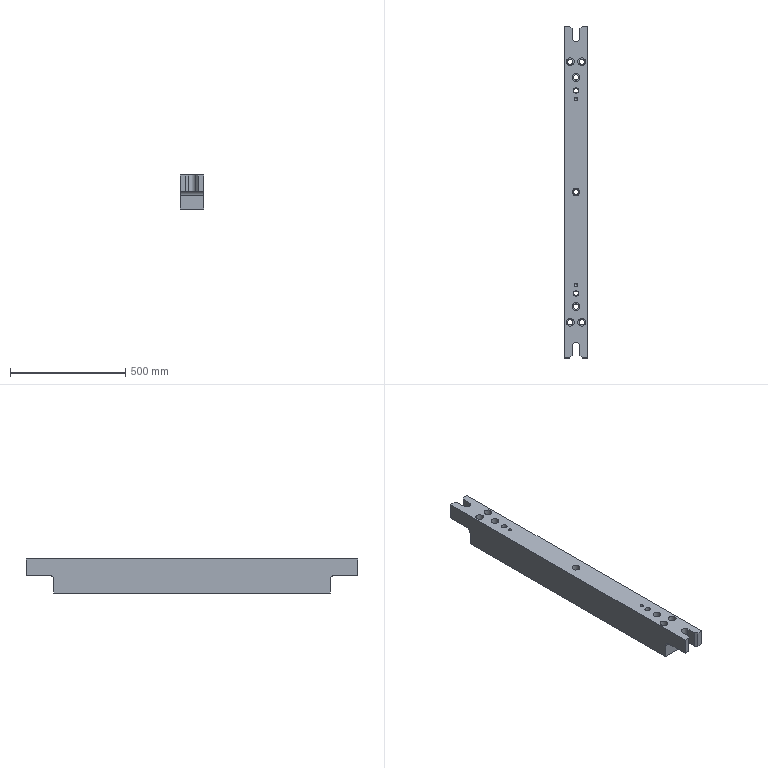Part | STEP file | lll_id1770_x_t | 1 solid | 55 faces | box 100 x 1440 x 147.5 mm | volume 18182535 mm3 | plane 29 | cylinder 24 | cone 2 | commonest cylinder face diameters 23.009 x7 34.008 x7 14.506 x2 20 x2 24 x2 34 x2
STEP:
#1=CARTESIAN_POINT('',(2475.431,565.,370.));
#2=VERTEX_POINT('',#1);
#3=CARTESIAN_POINT('',(2492.435,565.,370.));
#4=DIRECTION('',(0.,0.,-1.));
#5=DIRECTION('',(-1.,0.,0.));
#6=AXIS2_PLACEMENT_3D('',#3,#4,#5);
#7=CIRCLE('',#6,17.004);
#8=EDGE_CURVE('',#2,#2,#7,.T.);
#9=ORIENTED_EDGE('',*,*,#8,.T.);
#10=EDGE_LOOP('',(#9));
#11=FACE_BOUND('',#10,.T.);
#12=CARTESIAN_POINT('',(2505.435,440.,370.));
#13=VERTEX_POINT('',#12);
#14=CARTESIAN_POINT('',(2517.435,440.,370.));
#15=DIRECTION('',(0.,0.,-1.));
#16=DIRECTION('',(-1.,0.,0.));
#17=AXIS2_PLACEMENT_3D('',#14,#15,#16);
#18=CIRCLE('',#17,12.);
#19=EDGE_CURVE('',#13,#13,#18,.T.);
#20=ORIENTED_EDGE('',*,*,#19,.T.);
#21=EDGE_LOOP('',(#20));
#22=FACE_BOUND('',#21,.T.);
#23=CARTESIAN_POINT('',(2500.431,497.,370.));
#24=VERTEX_POINT('',#23);
#25=CARTESIAN_POINT('',(2517.435,497.,370.));
#26=DIRECTION('',(0.,0.,-1.));
#27=DIRECTION('',(-1.,0.,0.));
#28=AXIS2_PLACEMENT_3D('',#25,#26,#27);
#29=CIRCLE('',#28,17.004);
#30=EDGE_CURVE('',#24,#24,#29,.T.);
#31=ORIENTED_EDGE('',*,*,#30,.T.);
#32=EDGE_LOOP('',(#31));
#33=FACE_BOUND('',#32,.T.);
#34=CARTESIAN_POINT('',(2525.431,565.,370.));
#35=VERTEX_POINT('',#34);
#36=CARTESIAN_POINT('',(2542.435,565.,370.));
#37=DIRECTION('',(0.,0.,-1.));
#38=DIRECTION('',(-1.,0.,0.));
#39=AXIS2_PLACEMENT_3D('',#36,#37,#38);
#40=CIRCLE('',#39,17.004);
#41=EDGE_CURVE('',#35,#35,#40,.T.);
#42=ORIENTED_EDGE('',*,*,#41,.T.);
#43=EDGE_LOOP('',(#42));
#44=FACE_BOUND('',#43,.T.);
#45=CARTESIAN_POINT('',(2534.439,0.,370.));
#46=VERTEX_POINT('',#45);
#47=CARTESIAN_POINT('',(2517.435,0.,370.));
#48=DIRECTION('',(0.,0.,-1.));
#49=DIRECTION('',(1.,0.,0.));
#50=AXIS2_PLACEMENT_3D('',#47,#48,#49);
#51=CIRCLE('',#50,17.004);
#52=EDGE_CURVE('',#46,#46,#51,.T.);
#53=ORIENTED_EDGE('',*,*,#52,.T.);
#54=EDGE_LOOP('',(#53));
#55=FACE_BOUND('',#54,.T.);
#56=CARTESIAN_POINT('',(2534.439,-497.,370.));
#57=VERTEX_POINT('',#56);
#58=CARTESIAN_POINT('',(2517.435,-497.,370.));
#59=DIRECTION('',(0.,0.,1.));
#60=DIRECTION('',(1.,0.,0.));
#61=AXIS2_PLACEMENT_3D('',#58,#59,#60);
#62=CIRCLE('',#61,17.004);
#63=EDGE_CURVE('',#57,#57,#62,.T.);
#64=ORIENTED_EDGE('',*,*,#63,.F.);
#65=EDGE_LOOP('',(#64));
#66=FACE_BOUND('',#65,.T.);
#67=CARTESIAN_POINT('',(2534.435,-710.,370.));
#68=VERTEX_POINT('',#67);
#69=CARTESIAN_POINT('',(2534.435,-670.,370.));
#70=VERTEX_POINT('',#69);
#71=CARTESIAN_POINT('',(2534.435,120.,370.));
#72=DIRECTION('',(0.,1.,0.));
#73=VECTOR('',#72,1.);
#74=LINE('',#71,#73);
#75=EDGE_CURVE('',#68,#70,#74,.T.);
#76=ORIENTED_EDGE('',*,*,#75,.F.);
#77=CARTESIAN_POINT('',(2544.435,-720.,370.));
#78=VERTEX_POINT('',#77);
#79=CARTESIAN_POINT('',(2534.435,-710.,370.));
#80=DIRECTION('',(0.7071,-0.7071,0.));
#81=VECTOR('',#80,1.);
#82=LINE('',#79,#81);
#83=EDGE_CURVE('',#68,#78,#82,.T.);
#84=ORIENTED_EDGE('',*,*,#83,.T.);
#85=CARTESIAN_POINT('',(2567.435,-720.,370.));
#86=VERTEX_POINT('',#85);
#87=CARTESIAN_POINT('',(301.12,-720.,370.));
#88=DIRECTION('',(-1.,0.,0.));
#89=VECTOR('',#88,1.);
#90=LINE('',#87,#89);
#91=EDGE_CURVE('',#86,#78,#90,.T.);
#92=ORIENTED_EDGE('',*,*,#91,.F.);
#93=CARTESIAN_POINT('',(2567.435,720.,370.));
#94=VERTEX_POINT('',#93);
#95=CARTESIAN_POINT('',(2567.435,0.,370.));
#96=DIRECTION('',(0.,-1.,0.));
#97=VECTOR('',#96,1.);
#98=LINE('',#95,#97);
#99=EDGE_CURVE('',#94,#86,#98,.T.);
#100=ORIENTED_EDGE('',*,*,#99,.F.);
#101=CARTESIAN_POINT('',(2544.435,720.,370.));
#102=VERTEX_POINT('',#101);
#103=CARTESIAN_POINT('',(301.12,720.,370.));
#104=DIRECTION('',(1.,0.,0.));
#105=VECTOR('',#104,1.);
#106=LINE('',#103,#105);
#107=EDGE_CURVE('',#102,#94,#106,.T.);
#108=ORIENTED_EDGE('',*,*,#107,.F.);
#109=CARTESIAN_POINT('',(2534.435,710.,370.));
#110=VERTEX_POINT('',#109);
#111=CARTESIAN_POINT('',(2500.935,676.5,370.));
#112=DIRECTION('',(0.7071,0.7071,0.));
#113=VECTOR('',#112,1.);
#114=LINE('',#111,#113);
#115=EDGE_CURVE('',#110,#102,#114,.T.);
#116=ORIENTED_EDGE('',*,*,#115,.F.);
#117=CARTESIAN_POINT('',(2534.435,670.,370.));
#118=VERTEX_POINT('',#117);
#119=CARTESIAN_POINT('',(2534.435,-120.,370.));
#120=DIRECTION('',(0.,-1.,0.));
#121=VECTOR('',#120,1.);
#122=LINE('',#119,#121);
#123=EDGE_CURVE('',#110,#118,#122,.T.);
#124=ORIENTED_EDGE('',*,*,#123,.T.);
#125=CARTESIAN_POINT('',(2500.435,670.,370.));
#126=VERTEX_POINT('',#125);
#127=CARTESIAN_POINT('',(2517.435,670.,370.));
#128=DIRECTION('',(0.,0.,-1.));
#129=DIRECTION('',(1.,0.,0.));
#130=AXIS2_PLACEMENT_3D('',#127,#128,#129);
#131=CIRCLE('',#130,17.);
#132=EDGE_CURVE('',#118,#126,#131,.T.);
#133=ORIENTED_EDGE('',*,*,#132,.T.);
#134=CARTESIAN_POINT('',(2500.435,710.,370.));
#135=VERTEX_POINT('',#134);
#136=CARTESIAN_POINT('',(2500.435,-120.,370.));
#137=DIRECTION('',(0.,1.,0.));
#138=VECTOR('',#137,1.);
#139=LINE('',#136,#138);
#140=EDGE_CURVE('',#126,#135,#139,.T.);
#141=ORIENTED_EDGE('',*,*,#140,.T.);
#142=CARTESIAN_POINT('',(2490.435,720.,370.));
#143=VERTEX_POINT('',#142);
#144=CARTESIAN_POINT('',(3193.935,16.5,370.));
#145=DIRECTION('',(0.7071,-0.7071,0.));
#146=VECTOR('',#145,1.);
#147=LINE('',#144,#146);
#148=EDGE_CURVE('',#143,#135,#147,.T.);
#149=ORIENTED_EDGE('',*,*,#148,.F.);
#150=CARTESIAN_POINT('',(2467.435,720.,370.));
#151=VERTEX_POINT('',#150);
#152=CARTESIAN_POINT('',(301.12,720.,370.));
#153=DIRECTION('',(1.,0.,0.));
#154=VECTOR('',#153,1.);
#155=LINE('',#152,#154);
#156=EDGE_CURVE('',#151,#143,#155,.T.);
#157=ORIENTED_EDGE('',*,*,#156,.F.);
#158=CARTESIAN_POINT('',(2467.435,-720.,370.));
#159=VERTEX_POINT('',#158);
#160=CARTESIAN_POINT('',(2467.435,-1.,370.));
#161=DIRECTION('',(0.,1.,0.));
#162=VECTOR('',#161,1.);
#163=LINE('',#160,#162);
#164=EDGE_CURVE('',#159,#151,#163,.T.);
#165=ORIENTED_EDGE('',*,*,#164,.F.);
#166=CARTESIAN_POINT('',(2490.435,-720.,370.));
#167=VERTEX_POINT('',#166);
#168=CARTESIAN_POINT('',(301.12,-720.,370.));
#169=DIRECTION('',(-1.,0.,0.));
#170=VECTOR('',#169,1.);
#171=LINE('',#168,#170);
#172=EDGE_CURVE('',#167,#159,#171,.T.);
#173=ORIENTED_EDGE('',*,*,#172,.F.);
#174=CARTESIAN_POINT('',(2500.435,-710.,370.));
#175=VERTEX_POINT('',#174);
#176=CARTESIAN_POINT('',(2500.435,-710.,370.));
#177=DIRECTION('',(0.7071,0.7071,0.));
#178=VECTOR('',#177,1.);
#179=LINE('',#176,#178);
#180=EDGE_CURVE('',#167,#175,#179,.T.);
#181=ORIENTED_EDGE('',*,*,#180,.T.);
#182=CARTESIAN_POINT('',(2500.435,-670.,370.));
#183=VERTEX_POINT('',#182);
#184=CARTESIAN_POINT('',(2500.435,120.,370.));
#185=DIRECTION('',(0.,-1.,0.));
#186=VECTOR('',#185,1.);
#187=LINE('',#184,#186);
#188=EDGE_CURVE('',#183,#175,#187,.T.);
#189=ORIENTED_EDGE('',*,*,#188,.F.);
#190=CARTESIAN_POINT('',(2517.435,-670.,370.));
#191=DIRECTION('',(0.,0.,1.));
#192=DIRECTION('',(1.,0.,0.));
#193=AXIS2_PLACEMENT_3D('',#190,#191,#192);
#194=CIRCLE('',#193,17.);
#195=EDGE_CURVE('',#70,#183,#194,.T.);
#196=ORIENTED_EDGE('',*,*,#195,.F.);
#197=EDGE_LOOP('',(#76,#84,#92,#100,#108,#116,#124,#133,#141,#149,#157,#165,#173,#181,#189,#196));
#198=FACE_BOUND('',#197,.T.);
#199=CARTESIAN_POINT('',(2505.435,-440.,370.));
#200=VERTEX_POINT('',#199);
#201=CARTESIAN_POINT('',(2517.435,-440.,370.));
#202=DIRECTION('',(0.,0.,-1.));
#203=DIRECTION('',(-1.,0.,0.));
#204=AXIS2_PLACEMENT_3D('',#201,#202,#203);
#205=CIRCLE('',#204,12.);
#206=EDGE_CURVE('',#200,#200,#205,.T.);
#207=ORIENTED_EDGE('',*,*,#206,.T.);
#208=EDGE_LOOP('',(#207));
#209=FACE_BOUND('',#208,.T.);
#210=CARTESIAN_POINT('',(2525.431,-565.,370.));
#211=VERTEX_POINT('',#210);
#212=CARTESIAN_POINT('',(2542.435,-565.,370.));
#213=DIRECTION('',(0.,0.,-1.));
#214=DIRECTION('',(-1.,0.,0.));
#215=AXIS2_PLACEMENT_3D('',#212,#213,#214);
#216=CIRCLE('',#215,17.004);
#217=EDGE_CURVE('',#211,#211,#216,.T.);
#218=ORIENTED_EDGE('',*,*,#217,.T.);
#219=EDGE_LOOP('',(#218));
#220=FACE_BOUND('',#219,.T.);
#221=CARTESIAN_POINT('',(2509.439,-565.,370.));
#222=VERTEX_POINT('',#221);
#223=CARTESIAN_POINT('',(2492.435,-565.,370.));
#224=DIRECTION('',(0.,0.,1.));
#225=DIRECTION('',(1.,0.,0.));
#226=AXIS2_PLACEMENT_3D('',#223,#224,#225);
#227=CIRCLE('',#226,17.004);
#228=EDGE_CURVE('',#222,#222,#227,.T.);
#229=ORIENTED_EDGE('',*,*,#228,.F.);
#230=EDGE_LOOP('',(#229));
#231=FACE_BOUND('',#230,.T.);
#232=CARTESIAN_POINT('',(2524.688,-403.,370.));
#233=VERTEX_POINT('',#232);
#234=CARTESIAN_POINT('',(2517.435,-403.,370.));
#235=DIRECTION('',(0.,0.,-1.));
#236=DIRECTION('',(1.,0.,0.));
#237=AXIS2_PLACEMENT_3D('',#234,#235,#236);
#238=CIRCLE('',#237,7.253);
#239=EDGE_CURVE('',#233,#233,#238,.T.);
#240=ORIENTED_EDGE('',*,*,#239,.T.);
#241=EDGE_LOOP('',(#240));
#242=FACE_BOUND('',#241,.T.);
#243=CARTESIAN_POINT('',(2524.688,403.,370.));
#244=VERTEX_POINT('',#243);
#245=CARTESIAN_POINT('',(2517.435,403.,370.));
#246=DIRECTION('',(0.,0.,1.));
#247=DIRECTION('',(1.,0.,0.));
#248=AXIS2_PLACEMENT_3D('',#245,#246,#247);
#249=CIRCLE('',#248,7.253);
#250=EDGE_CURVE('',#244,#244,#249,.T.);
#251=ORIENTED_EDGE('',*,*,#250,.F.);
#252=EDGE_LOOP('',(#251));
#253=FACE_BOUND('',#252,.T.);
#254=CARTESIAN_POINT('',(301.12,-1.,370.));
#255=DIRECTION('',(0.,0.,-1.));
#256=DIRECTION('',(1.,0.,0.));
#257=AXIS2_PLACEMENT_3D('',#254,#255,#256);
#258=PLANE('',#257);
#259=ADVANCED_FACE('',(#11,#22,#33,#44,#55,#66,#198,#209,#220,#231,#242,#253),#258,.F.);
#260=CARTESIAN_POINT('',(2567.435,600.,280.));
#261=VERTEX_POINT('',#260);
#262=CARTESIAN_POINT('',(2567.435,620.,300.));
#263=VERTEX_POINT('',#262);
#264=CARTESIAN_POINT('',(2567.435,620.,280.));
#265=DIRECTION('',(-1.,0.,0.));
#266=DIRECTION('',(0.,0.,-1.));
#267=AXIS2_PLACEMENT_3D('',#264,#265,#266);
#268=CIRCLE('',#267,20.);
#269=EDGE_CURVE('',#261,#263,#268,.T.);
#270=ORIENTED_EDGE('',*,*,#269,.F.);
#271=CARTESIAN_POINT('',(2467.435,600.,280.));
#272=VERTEX_POINT('',#271);
#273=CARTESIAN_POINT('',(2557.435,600.,280.));
#274=DIRECTION('',(1.,0.,0.));
#275=VECTOR('',#274,1.);
#276=LINE('',#273,#275);
#277=EDGE_CURVE('',#272,#261,#276,.T.);
#278=ORIENTED_EDGE('',*,*,#277,.F.);
#279=CARTESIAN_POINT('',(2467.435,620.,300.));
#280=VERTEX_POINT('',#279);
#281=CARTESIAN_POINT('',(2467.435,620.,280.));
#282=DIRECTION('',(1.,0.,0.));
#283=DIRECTION('',(0.,0.,-1.));
#284=AXIS2_PLACEMENT_3D('',#281,#282,#283);
#285=CIRCLE('',#284,20.);
#286=EDGE_CURVE('',#280,#272,#285,.T.);
#287=ORIENTED_EDGE('',*,*,#286,.F.);
#288=CARTESIAN_POINT('',(2477.435,620.,300.));
#289=DIRECTION('',(-1.,0.,0.));
#290=VECTOR('',#289,1.);
#291=LINE('',#288,#290);
#292=EDGE_CURVE('',#263,#280,#291,.T.);
#293=ORIENTED_EDGE('',*,*,#292,.F.);
#294=EDGE_LOOP('',(#270,#278,#287,#293));
#295=FACE_OUTER_BOUND('',#294,.T.);
#296=CARTESIAN_POINT('',(2517.435,620.,280.));
#297=DIRECTION('',(1.,0.,0.));
#298=DIRECTION('',(0.,0.,1.));
#299=AXIS2_PLACEMENT_3D('',#296,#297,#298);
#300=CYLINDRICAL_SURFACE('',#299,20.);
#301=ADVANCED_FACE('',(#295),#300,.F.);
#302=CARTESIAN_POINT('',(2567.435,720.,300.));
#303=VERTEX_POINT('',#302);
#304=CARTESIAN_POINT('',(2567.435,-641.5,300.));
#305=DIRECTION('',(0.,1.,0.));
#306=VECTOR('',#305,1.);
#307=LINE('',#304,#306);
#308=EDGE_CURVE('',#263,#303,#307,.T.);
#309=ORIENTED_EDGE('',*,*,#308,.F.);
#310=ORIENTED_EDGE('',*,*,#292,.T.);
#311=CARTESIAN_POINT('',(2467.435,720.,300.));
#312=VERTEX_POINT('',#311);
#313=CARTESIAN_POINT('',(2467.435,-641.5,300.));
#314=DIRECTION('',(0.,1.,0.));
#315=VECTOR('',#314,1.);
#316=LINE('',#313,#315);
#317=EDGE_CURVE('',#280,#312,#316,.T.);
#318=ORIENTED_EDGE('',*,*,#317,.T.);
#319=CARTESIAN_POINT('',(2490.435,720.,300.));
#320=VERTEX_POINT('',#319);
#321=CARTESIAN_POINT('',(2517.435,720.,300.));
#322=DIRECTION('',(1.,0.,0.));
#323=VECTOR('',#322,1.);
#324=LINE('',#321,#323);
#325=EDGE_CURVE('',#312,#320,#324,.T.);
#326=ORIENTED_EDGE('',*,*,#325,.T.);
#327=CARTESIAN_POINT('',(2500.435,710.,300.));
#328=VERTEX_POINT('',#327);
#329=CARTESIAN_POINT('',(2490.435,720.,300.));
#330=DIRECTION('',(0.7071,-0.7071,0.));
#331=VECTOR('',#330,1.);
#332=LINE('',#329,#331);
#333=EDGE_CURVE('',#320,#328,#332,.T.);
#334=ORIENTED_EDGE('',*,*,#333,.T.);
#335=CARTESIAN_POINT('',(2500.435,670.,300.));
#336=VERTEX_POINT('',#335);
#337=CARTESIAN_POINT('',(2500.435,-641.5,300.));
#338=DIRECTION('',(0.,-1.,0.));
#339=VECTOR('',#338,1.);
#340=LINE('',#337,#339);
#341=EDGE_CURVE('',#328,#336,#340,.T.);
#342=ORIENTED_EDGE('',*,*,#341,.T.);
#343=CARTESIAN_POINT('',(2534.435,670.,300.));
#344=VERTEX_POINT('',#343);
#345=CARTESIAN_POINT('',(2517.435,670.,300.));
#346=DIRECTION('',(0.,0.,-1.));
#347=DIRECTION('',(-1.,0.,0.));
#348=AXIS2_PLACEMENT_3D('',#345,#346,#347);
#349=CIRCLE('',#348,17.);
#350=EDGE_CURVE('',#344,#336,#349,.T.);
#351=ORIENTED_EDGE('',*,*,#350,.F.);
#352=CARTESIAN_POINT('',(2534.435,710.,300.));
#353=VERTEX_POINT('',#352);
#354=CARTESIAN_POINT('',(2534.435,-641.5,300.));
#355=DIRECTION('',(0.,1.,0.));
#356=VECTOR('',#355,1.);
#357=LINE('',#354,#356);
#358=EDGE_CURVE('',#344,#353,#357,.T.);
#359=ORIENTED_EDGE('',*,*,#358,.T.);
#360=CARTESIAN_POINT('',(2544.435,720.,300.));
#361=VERTEX_POINT('',#360);
#362=CARTESIAN_POINT('',(2544.435,720.,300.));
#363=DIRECTION('',(0.7071,0.7071,0.));
#364=VECTOR('',#363,1.);
#365=LINE('',#362,#364);
#366=EDGE_CURVE('',#353,#361,#365,.T.);
#367=ORIENTED_EDGE('',*,*,#366,.T.);
#368=CARTESIAN_POINT('',(2517.435,720.,300.));
#369=DIRECTION('',(1.,0.,0.));
#370=VECTOR('',#369,1.);
#371=LINE('',#368,#370);
#372=EDGE_CURVE('',#361,#303,#371,.T.);
#373=ORIENTED_EDGE('',*,*,#372,.T.);
#374=EDGE_LOOP('',(#309,#310,#318,#326,#334,#342,#351,#359,#367,#373));
#375=FACE_OUTER_BOUND('',#374,.T.);
#376=CARTESIAN_POINT('',(2517.435,-641.5,300.));
#377=DIRECTION('',(0.,0.,-1.));
#378=DIRECTION('',(1.,0.,0.));
#379=AXIS2_PLACEMENT_3D('',#376,#377,#378);
#380=PLANE('',#379);
#381=ADVANCED_FACE('',(#375),#380,.T.);
#382=CARTESIAN_POINT('',(2567.435,-720.,300.));
#383=VERTEX_POINT('',#382);
#384=CARTESIAN_POINT('',(2544.435,-720.,300.));
#385=VERTEX_POINT('',#384);
#386=CARTESIAN_POINT('',(2517.435,-720.,300.));
#387=DIRECTION('',(-1.,0.,0.));
#388=VECTOR('',#387,1.);
#389=LINE('',#386,#388);
#390=EDGE_CURVE('',#383,#385,#389,.T.);
#391=ORIENTED_EDGE('',*,*,#390,.T.);
#392=CARTESIAN_POINT('',(2534.435,-710.,300.));
#393=VERTEX_POINT('',#392);
#394=CARTESIAN_POINT('',(2511.685,-687.25,300.));
#395=DIRECTION('',(-0.7071,0.7071,0.));
#396=VECTOR('',#395,1.);
#397=LINE('',#394,#396);
#398=EDGE_CURVE('',#385,#393,#397,.T.);
#399=ORIENTED_EDGE('',*,*,#398,.T.);
#400=CARTESIAN_POINT('',(2534.435,-670.,300.));
#401=VERTEX_POINT('',#400);
#402=CARTESIAN_POINT('',(2534.435,-661.5,300.));
#403=DIRECTION('',(0.,-1.,0.));
#404=VECTOR('',#403,1.);
#405=LINE('',#402,#404);
#406=EDGE_CURVE('',#401,#393,#405,.T.);
#407=ORIENTED_EDGE('',*,*,#406,.F.);
#408=CARTESIAN_POINT('',(2500.435,-670.,300.));
#409=VERTEX_POINT('',#408);
#410=CARTESIAN_POINT('',(2517.435,-670.,300.));
#411=DIRECTION('',(0.,0.,1.));
#412=DIRECTION('',(1.,0.,0.));
#413=AXIS2_PLACEMENT_3D('',#410,#411,#412);
#414=CIRCLE('',#413,17.);
#415=EDGE_CURVE('',#401,#409,#414,.T.);
#416=ORIENTED_EDGE('',*,*,#415,.T.);
#417=CARTESIAN_POINT('',(2500.435,-710.,300.));
#418=VERTEX_POINT('',#417);
#419=CARTESIAN_POINT('',(2500.435,-661.5,300.));
#420=DIRECTION('',(0.,1.,0.));
#421=VECTOR('',#420,1.);
#422=LINE('',#419,#421);
#423=EDGE_CURVE('',#418,#409,#422,.T.);
#424=ORIENTED_EDGE('',*,*,#423,.F.);
#425=CARTESIAN_POINT('',(2490.435,-720.,300.));
#426=VERTEX_POINT('',#425);
#427=CARTESIAN_POINT('',(2523.185,-687.25,300.));
#428=DIRECTION('',(-0.7071,-0.7071,0.));
#429=VECTOR('',#428,1.);
#430=LINE('',#427,#429);
#431=EDGE_CURVE('',#418,#426,#430,.T.);
#432=ORIENTED_EDGE('',*,*,#431,.T.);
#433=CARTESIAN_POINT('',(2467.435,-720.,300.));
#434=VERTEX_POINT('',#433);
#435=CARTESIAN_POINT('',(2517.435,-720.,300.));
#436=DIRECTION('',(-1.,0.,0.));
#437=VECTOR('',#436,1.);
#438=LINE('',#435,#437);
#439=EDGE_CURVE('',#426,#434,#438,.T.);
#440=ORIENTED_EDGE('',*,*,#439,.T.);
#441=CARTESIAN_POINT('',(2467.435,-620.,300.));
#442=VERTEX_POINT('',#441);
#443=CARTESIAN_POINT('',(2467.435,-681.5,300.));
#444=DIRECTION('',(0.,1.,0.));
#445=VECTOR('',#444,1.);
#446=LINE('',#443,#445);
#447=EDGE_CURVE('',#434,#442,#446,.T.);
#448=ORIENTED_EDGE('',*,*,#447,.T.);
#449=CARTESIAN_POINT('',(2567.435,-620.,300.));
#450=VERTEX_POINT('',#449);
#451=CARTESIAN_POINT('',(2557.435,-620.,300.));
#452=DIRECTION('',(1.,0.,0.));
#453=VECTOR('',#452,1.);
#454=LINE('',#451,#453);
#455=EDGE_CURVE('',#442,#450,#454,.T.);
#456=ORIENTED_EDGE('',*,*,#455,.T.);
#457=CARTESIAN_POINT('',(2567.435,-681.5,300.));
#458=DIRECTION('',(0.,1.,0.));
#459=VECTOR('',#458,1.);
#460=LINE('',#457,#459);
#461=EDGE_CURVE('',#383,#450,#460,.T.);
#462=ORIENTED_EDGE('',*,*,#461,.F.);
#463=EDGE_LOOP('',(#391,#399,#407,#416,#424,#432,#440,#448,#456,#462));
#464=FACE_OUTER_BOUND('',#463,.T.);
#465=CARTESIAN_POINT('',(2517.435,-681.5,300.));
#466=DIRECTION('',(0.,0.,-1.));
#467=DIRECTION('',(1.,0.,0.));
#468=AXIS2_PLACEMENT_3D('',#465,#466,#467);
#469=PLANE('',#468);
#470=ADVANCED_FACE('',(#464),#469,.T.);
#471=CARTESIAN_POINT('',(2467.435,-600.,280.));
#472=VERTEX_POINT('',#471);
#473=CARTESIAN_POINT('',(2467.435,-620.,280.));
#474=DIRECTION('',(1.,0.,0.));
#475=DIRECTION('',(0.,0.,-1.));
#476=AXIS2_PLACEMENT_3D('',#473,#474,#475);
#477=CIRCLE('',#476,20.);
#478=EDGE_CURVE('',#472,#442,#477,.T.);
#479=ORIENTED_EDGE('',*,*,#478,.F.);
#480=CARTESIAN_POINT('',(2567.435,-600.,280.));
#481=VERTEX_POINT('',#480);
#482=CARTESIAN_POINT('',(2477.435,-600.,280.));
#483=DIRECTION('',(-1.,0.,0.));
#484=VECTOR('',#483,1.);
#485=LINE('',#482,#484);
#486=EDGE_CURVE('',#481,#472,#485,.T.);
#487=ORIENTED_EDGE('',*,*,#486,.F.);
#488=CARTESIAN_POINT('',(2567.435,-620.,280.));
#489=DIRECTION('',(-1.,0.,0.));
#490=DIRECTION('',(0.,0.,-1.));
#491=AXIS2_PLACEMENT_3D('',#488,#489,#490);
#492=CIRCLE('',#491,20.);
#493=EDGE_CURVE('',#450,#481,#492,.T.);
#494=ORIENTED_EDGE('',*,*,#493,.F.);
#495=ORIENTED_EDGE('',*,*,#455,.F.);
#496=EDGE_LOOP('',(#479,#487,#494,#495));
#497=FACE_OUTER_BOUND('',#496,.T.);
#498=CARTESIAN_POINT('',(2517.435,-620.,280.));
#499=DIRECTION('',(-1.,0.,0.));
#500=DIRECTION('',(0.,0.,-1.));
#501=AXIS2_PLACEMENT_3D('',#498,#499,#500);
#502=CYLINDRICAL_SURFACE('',#501,20.);
#503=ADVANCED_FACE('',(#497),#502,.F.);
#504=CARTESIAN_POINT('',(2505.435,-440.,270.));
#505=VERTEX_POINT('',#504);
#506=CARTESIAN_POINT('',(2517.435,-440.,270.));
#507=DIRECTION('',(0.,0.,-1.));
#508=DIRECTION('',(-1.,0.,0.));
#509=AXIS2_PLACEMENT_3D('',#506,#507,#508);
#510=CIRCLE('',#509,12.);
#511=EDGE_CURVE('',#505,#505,#510,.T.);
#512=ORIENTED_EDGE('',*,*,#511,.F.);
#513=EDGE_LOOP('',(#512));
#514=FACE_BOUND('',#513,.T.);
#515=CARTESIAN_POINT('',(2527.435,-440.,270.));
#516=VERTEX_POINT('',#515);
#517=CARTESIAN_POINT('',(2517.435,-440.,270.));
#518=DIRECTION('',(0.,0.,1.));
#519=DIRECTION('',(1.,0.,0.));
#520=AXIS2_PLACEMENT_3D('',#517,#518,#519);
#521=CIRCLE('',#520,10.);
#522=EDGE_CURVE('',#516,#516,#521,.T.);
#523=ORIENTED_EDGE('',*,*,#522,.F.);
#524=EDGE_LOOP('',(#523));
#525=FACE_BOUND('',#524,.T.);
#526=CARTESIAN_POINT('',(2517.435,-440.,270.));
#527=DIRECTION('',(0.,0.,-1.));
#528=DIRECTION('',(1.,0.,0.));
#529=AXIS2_PLACEMENT_3D('',#526,#527,#528);
#530=PLANE('',#529);
#531=ADVANCED_FACE('',(#514,#525),#530,.F.);
#532=CARTESIAN_POINT('',(2553.94,-565.,272.5));
#533=VERTEX_POINT('',#532);
#534=CARTESIAN_POINT('',(2542.435,-565.,272.5));
#535=DIRECTION('',(0.,0.,-1.));
#536=DIRECTION('',(1.,0.,0.));
#537=AXIS2_PLACEMENT_3D('',#534,#535,#536);
#538=CIRCLE('',#537,11.505);
#539=EDGE_CURVE('',#533,#533,#538,.T.);
#540=ORIENTED_EDGE('',*,*,#539,.T.);
#541=EDGE_LOOP('',(#540));
#542=FACE_BOUND('',#541,.T.);
#543=CARTESIAN_POINT('',(2525.431,-565.,272.5));
#544=VERTEX_POINT('',#543);
#545=CARTESIAN_POINT('',(2542.435,-565.,272.5));
#546=DIRECTION('',(0.,0.,-1.));
#547=DIRECTION('',(-1.,0.,0.));
#548=AXIS2_PLACEMENT_3D('',#545,#546,#547);
#549=CIRCLE('',#548,17.004);
#550=EDGE_CURVE('',#544,#544,#549,.T.);
#551=ORIENTED_EDGE('',*,*,#550,.F.);
#552=EDGE_LOOP('',(#551));
#553=FACE_BOUND('',#552,.T.);
#554=CARTESIAN_POINT('',(2542.435,-565.,272.5));
#555=DIRECTION('',(0.,0.,-1.));
#556=DIRECTION('',(1.,0.,0.));
#557=AXIS2_PLACEMENT_3D('',#554,#555,#556);
#558=PLANE('',#557);
#559=ADVANCED_FACE('',(#542,#553),#558,.F.);
#560=CARTESIAN_POINT('',(2480.931,-565.,272.5));
#561=VERTEX_POINT('',#560);
#562=CARTESIAN_POINT('',(2492.435,-565.,272.5));
#563=DIRECTION('',(0.,0.,1.));
#564=DIRECTION('',(-1.,0.,0.));
#565=AXIS2_PLACEMENT_3D('',#562,#563,#564);
#566=CIRCLE('',#565,11.505);
#567=EDGE_CURVE('',#561,#561,#566,.T.);
#568=ORIENTED_EDGE('',*,*,#567,.F.);
#569=EDGE_LOOP('',(#568));
#570=FACE_BOUND('',#569,.T.);
#571=CARTESIAN_POINT('',(2509.439,-565.,272.5));
#572=VERTEX_POINT('',#571);
#573=CARTESIAN_POINT('',(2492.435,-565.,272.5));
#574=DIRECTION('',(0.,0.,1.));
#575=DIRECTION('',(1.,0.,0.));
#576=AXIS2_PLACEMENT_3D('',#573,#574,#575);
#577=CIRCLE('',#576,17.004);
#578=EDGE_CURVE('',#572,#572,#577,.T.);
#579=ORIENTED_EDGE('',*,*,#578,.T.);
#580=EDGE_LOOP('',(#579));
#581=FACE_BOUND('',#580,.T.);
#582=CARTESIAN_POINT('',(2492.435,-565.,272.5));
#583=DIRECTION('',(0.,0.,-1.));
#584=DIRECTION('',(-1.,0.,0.));
#585=AXIS2_PLACEMENT_3D('',#582,#583,#584);
#586=PLANE('',#585);
#587=ADVANCED_FACE('',(#570,#581),#586,.F.);
#588=CARTESIAN_POINT('',(2505.931,-497.,272.5));
#589=VERTEX_POINT('',#588);
#590=CARTESIAN_POINT('',(2517.435,-497.,272.5));
#591=DIRECTION('',(0.,0.,1.));
#592=DIRECTION('',(-1.,0.,0.));
#593=AXIS2_PLACEMENT_3D('',#590,#591,#592);
#594=CIRCLE('',#593,11.505);
#595=EDGE_CURVE('',#589,#589,#594,.T.);
#596=ORIENTED_EDGE('',*,*,#595,.F.);
#597=EDGE_LOOP('',(#596));
#598=FACE_BOUND('',#597,.T.);
#599=CARTESIAN_POINT('',(2534.439,-497.,272.5));
#600=VERTEX_POINT('',#599);
#601=CARTESIAN_POINT('',(2517.435,-497.,272.5));
#602=DIRECTION('',(0.,0.,1.));
#603=DIRECTION('',(1.,0.,0.));
#604=AXIS2_PLACEMENT_3D('',#601,#602,#603);
#605=CIRCLE('',#604,17.004);
#606=EDGE_CURVE('',#600,#600,#605,.T.);
#607=ORIENTED_EDGE('',*,*,#606,.T.);
#608=EDGE_LOOP('',(#607));
#609=FACE_BOUND('',#608,.T.);
#610=CARTESIAN_POINT('',(2517.435,-497.,272.5));
#611=DIRECTION('',(0.,0.,-1.));
#612=DIRECTION('',(-1.,0.,0.));
#613=AXIS2_PLACEMENT_3D('',#610,#611,#612);
#614=PLANE('',#613);
#615=ADVANCED_FACE('',(#598,#609),#614,.F.);
#616=CARTESIAN_POINT('',(2505.931,0.,272.5));
#617=VERTEX_POINT('',#616);
#618=CARTESIAN_POINT('',(2517.435,0.,272.5));
#619=DIRECTION('',(0.,0.,-1.));
#620=DIRECTION('',(-1.,0.,0.));
#621=AXIS2_PLACEMENT_3D('',#618,#619,#620);
#622=CIRCLE('',#621,11.505);
#623=EDGE_CURVE('',#617,#617,#622,.T.);
#624=ORIENTED_EDGE('',*,*,#623,.T.);
#625=EDGE_LOOP('',(#624));
#626=FACE_BOUND('',#625,.T.);
#627=CARTESIAN_POINT('',(2534.439,0.,272.5));
#628=VERTEX_POINT('',#627);
#629=CARTESIAN_POINT('',(2517.435,0.,272.5));
#630=DIRECTION('',(0.,0.,-1.));
#631=DIRECTION('',(1.,0.,0.));
#632=AXIS2_PLACEMENT_3D('',#629,#630,#631);
#633=CIRCLE('',#632,17.004);
#634=EDGE_CURVE('',#628,#628,#633,.T.);
#635=ORIENTED_EDGE('',*,*,#634,.F.);
#636=EDGE_LOOP('',(#635));
#637=FACE_BOUND('',#636,.T.);
#638=CARTESIAN_POINT('',(2517.435,20.,272.5));
#639=DIRECTION('',(0.,0.,-1.));
#640=DIRECTION('',(-1.,0.,0.));
#641=AXIS2_PLACEMENT_3D('',#638,#639,#640);
#642=PLANE('',#641);
#643=ADVANCED_FACE('',(#626,#637),#642,.F.);
#644=ORIENTED_EDGE('',*,*,#578,.F.);
#645=EDGE_LOOP('',(#644));
#646=FACE_BOUND('',#645,.T.);
#647=ORIENTED_EDGE('',*,*,#228,.T.);
#648=EDGE_LOOP('',(#647));
#649=FACE_BOUND('',#648,.T.);
#650=CARTESIAN_POINT('',(2492.435,-565.,370.));
#651=DIRECTION('',(0.,0.,-1.));
#652=DIRECTION('',(1.,0.,0.));
#653=AXIS2_PLACEMENT_3D('',#650,#651,#652);
#654=CYLINDRICAL_SURFACE('',#653,17.004);
#655=ADVANCED_FACE('',(#646,#649),#654,.F.);
#656=ORIENTED_EDGE('',*,*,#550,.T.);
#657=EDGE_LOOP('',(#656));
#658=FACE_BOUND('',#657,.T.);
#659=ORIENTED_EDGE('',*,*,#217,.F.);
#660=EDGE_LOOP('',(#659));
#661=FACE_BOUND('',#660,.T.);
#662=CARTESIAN_POINT('',(2542.435,-565.,370.));
#663=DIRECTION('',(0.,0.,-1.));
#664=DIRECTION('',(-1.,0.,0.));
#665=AXIS2_PLACEMENT_3D('',#662,#663,#664);
#666=CYLINDRICAL_SURFACE('',#665,17.004);
#667=ADVANCED_FACE('',(#658,#661),#666,.F.);
#668=ORIENTED_EDGE('',*,*,#511,.T.);
#669=EDGE_LOOP('',(#668));
#670=FACE_BOUND('',#669,.T.);
#671=ORIENTED_EDGE('',*,*,#206,.F.);
#672=EDGE_LOOP('',(#671));
#673=FACE_BOUND('',#672,.T.);
#674=CARTESIAN_POINT('',(2517.435,-440.,370.));
#675=DIRECTION('',(0.,0.,-1.));
#676=DIRECTION('',(-1.,0.,0.));
#677=AXIS2_PLACEMENT_3D('',#674,#675,#676);
#678=CYLINDRICAL_SURFACE('',#677,12.);
#679=ADVANCED_FACE('',(#670,#673),#678,.F.);
#680=ORIENTED_EDGE('',*,*,#140,.F.);
#681=CARTESIAN_POINT('',(2500.435,670.,370.));
#682=DIRECTION('',(0.,0.,-1.));
#683=VECTOR('',#682,1.);
#684=LINE('',#681,#683);
#685=EDGE_CURVE('',#126,#336,#684,.T.);
#686=ORIENTED_EDGE('',*,*,#685,.T.);
#687=ORIENTED_EDGE('',*,*,#341,.F.);
#688=CARTESIAN_POINT('',(2500.435,710.,385.));
#689=DIRECTION('',(0.,0.,-1.));
#690=VECTOR('',#689,1.);
#691=LINE('',#688,#690);
#692=EDGE_CURVE('',#135,#328,#691,.T.);
#693=ORIENTED_EDGE('',*,*,#692,.F.);
#694=EDGE_LOOP('',(#680,#686,#687,#693));
#695=FACE_OUTER_BOUND('',#694,.T.);
#696=CARTESIAN_POINT('',(2500.435,-720.,385.));
#697=DIRECTION('',(1.,0.,0.));
#698=DIRECTION('',(0.,0.,-1.));
#699=AXIS2_PLACEMENT_3D('',#696,#697,#698);
#700=PLANE('',#699);
#701=ADVANCED_FACE('',(#695),#700,.T.);
#702=ORIENTED_EDGE('',*,*,#685,.F.);
#703=ORIENTED_EDGE('',*,*,#132,.F.);
#704=CARTESIAN_POINT('',(2534.435,670.,370.));
#705=DIRECTION('',(0.,0.,1.));
#706=VECTOR('',#705,1.);
#707=LINE('',#704,#706);
#708=EDGE_CURVE('',#344,#118,#707,.T.);
#709=ORIENTED_EDGE('',*,*,#708,.F.);
#710=ORIENTED_EDGE('',*,*,#350,.T.);
#711=EDGE_LOOP('',(#702,#703,#709,#710));
#712=FACE_OUTER_BOUND('',#711,.T.);
#713=CARTESIAN_POINT('',(2517.435,670.,345.));
#714=DIRECTION('',(0.,0.,-1.));
#715=DIRECTION('',(-1.,0.,0.));
#716=AXIS2_PLACEMENT_3D('',#713,#714,#715);
#717=CYLINDRICAL_SURFACE('',#716,17.);
#718=ADVANCED_FACE('',(#712),#717,.F.);
#719=ORIENTED_EDGE('',*,*,#358,.F.);
#720=ORIENTED_EDGE('',*,*,#708,.T.);
#721=ORIENTED_EDGE('',*,*,#123,.F.);
#722=CARTESIAN_POINT('',(2534.435,710.,385.));
#723=DIRECTION('',(0.,0.,1.));
#724=VECTOR('',#723,1.);
#725=LINE('',#722,#724);
#726=EDGE_CURVE('',#353,#110,#725,.T.);
#727=ORIENTED_EDGE('',*,*,#726,.F.);
#728=EDGE_LOOP('',(#719,#720,#721,#727));
#729=FACE_OUTER_BOUND('',#728,.T.);
#730=CARTESIAN_POINT('',(2534.435,-720.,385.));
#731=DIRECTION('',(-1.,0.,0.));
#732=DIRECTION('',(0.,0.,1.));
#733=AXIS2_PLACEMENT_3D('',#730,#731,#732);
#734=PLANE('',#733);
#735=ADVANCED_FACE('',(#729),#734,.T.);
#736=ORIENTED_EDGE('',*,*,#115,.T.);
#737=CARTESIAN_POINT('',(2544.435,720.,-450.));
#738=DIRECTION('',(0.,0.,-1.));
#739=VECTOR('',#738,1.);
#740=LINE('',#737,#739);
#741=EDGE_CURVE('',#102,#361,#740,.T.);
#742=ORIENTED_EDGE('',*,*,#741,.T.);
#743=ORIENTED_EDGE('',*,*,#366,.F.);
#744=ORIENTED_EDGE('',*,*,#726,.T.);
#745=EDGE_LOOP('',(#736,#742,#743,#744));
#746=FACE_OUTER_BOUND('',#745,.T.);
#747=CARTESIAN_POINT('',(2544.435,720.,-450.));
#748=DIRECTION('',(0.7071,-0.7071,0.));
#749=DIRECTION('',(0.,0.,-1.));
#750=AXIS2_PLACEMENT_3D('',#747,#748,#749);
#751=PLANE('',#750);
#752=ADVANCED_FACE('',(#746),#751,.F.);
#753=ORIENTED_EDGE('',*,*,#741,.F.);
#754=ORIENTED_EDGE('',*,*,#107,.T.);
#755=CARTESIAN_POINT('',(2567.435,720.,241.25));
#756=DIRECTION('',(0.,0.,-1.));
#757=VECTOR('',#756,1.);
#758=LINE('',#755,#757);
#759=EDGE_CURVE('',#94,#303,#758,.T.);
#760=ORIENTED_EDGE('',*,*,#759,.T.);
#761=ORIENTED_EDGE('',*,*,#372,.F.);
#762=EDGE_LOOP('',(#753,#754,#760,#761));
#763=FACE_OUTER_BOUND('',#762,.T.);
#764=CARTESIAN_POINT('',(2487.435,720.,310.));
#765=DIRECTION('',(0.,1.,0.));
#766=DIRECTION('',(0.,0.,-1.));
#767=AXIS2_PLACEMENT_3D('',#764,#765,#766);
#768=PLANE('',#767);
#769=ADVANCED_FACE('',(#763),#768,.T.);
#770=ORIENTED_EDGE('',*,*,#91,.T.);
#771=CARTESIAN_POINT('',(2544.435,-720.,310.));
#772=DIRECTION('',(0.,0.,-1.));
#773=VECTOR('',#772,1.);
#774=LINE('',#771,#773);
#775=EDGE_CURVE('',#78,#385,#774,.T.);
#776=ORIENTED_EDGE('',*,*,#775,.T.);
#777=ORIENTED_EDGE('',*,*,#390,.F.);
#778=CARTESIAN_POINT('',(2567.435,-720.,241.25));
#779=DIRECTION('',(0.,0.,1.));
#780=VECTOR('',#779,1.);
#781=LINE('',#778,#780);
#782=EDGE_CURVE('',#383,#86,#781,.T.);
#783=ORIENTED_EDGE('',*,*,#782,.T.);
#784=EDGE_LOOP('',(#770,#776,#777,#783));
#785=FACE_OUTER_BOUND('',#784,.T.);
#786=CARTESIAN_POINT('',(6457.435,-720.,310.));
#787=DIRECTION('',(0.,-1.,0.));
#788=DIRECTION('',(0.,0.,1.));
#789=AXIS2_PLACEMENT_3D('',#786,#787,#788);
#790=PLANE('',#789);
#791=ADVANCED_FACE('',(#785),#790,.T.);
#792=ORIENTED_EDGE('',*,*,#406,.T.);
#793=CARTESIAN_POINT('',(2534.435,-710.,385.));
#794=DIRECTION('',(0.,0.,1.));
#795=VECTOR('',#794,1.);
#796=LINE('',#793,#795);
#797=EDGE_CURVE('',#393,#68,#796,.T.);
#798=ORIENTED_EDGE('',*,*,#797,.T.);
#799=ORIENTED_EDGE('',*,*,#75,.T.);
#800=CARTESIAN_POINT('',(2534.435,-670.,370.));
#801=DIRECTION('',(0.,0.,1.));
#802=VECTOR('',#801,1.);
#803=LINE('',#800,#802);
#804=EDGE_CURVE('',#401,#70,#803,.T.);
#805=ORIENTED_EDGE('',*,*,#804,.F.);
#806=EDGE_LOOP('',(#792,#798,#799,#805));
#807=FACE_OUTER_BOUND('',#806,.T.);
#808=CARTESIAN_POINT('',(2534.435,720.,385.));
#809=DIRECTION('',(-1.,0.,0.));
#810=DIRECTION('',(0.,0.,1.));
#811=AXIS2_PLACEMENT_3D('',#808,#809,#810);
#812=PLANE('',#811);
#813=ADVANCED_FACE('',(#807),#812,.T.);
#814=CARTESIAN_POINT('',(2500.435,-670.,370.));
#815=DIRECTION('',(0.,0.,-1.));
#816=VECTOR('',#815,1.);
#817=LINE('',#814,#816);
#818=EDGE_CURVE('',#183,#409,#817,.T.);
#819=ORIENTED_EDGE('',*,*,#818,.T.);
#820=ORIENTED_EDGE('',*,*,#415,.F.);
#821=ORIENTED_EDGE('',*,*,#804,.T.);
#822=ORIENTED_EDGE('',*,*,#195,.T.);
#823=EDGE_LOOP('',(#819,#820,#821,#822));
#824=FACE_OUTER_BOUND('',#823,.T.);
#825=CARTESIAN_POINT('',(2517.435,-670.,345.));
#826=DIRECTION('',(0.,0.,-1.));
#827=DIRECTION('',(-1.,0.,0.));
#828=AXIS2_PLACEMENT_3D('',#825,#826,#827);
#829=CYLINDRICAL_SURFACE('',#828,17.);
#830=ADVANCED_FACE('',(#824),#829,.F.);
#831=ORIENTED_EDGE('',*,*,#188,.T.);
#832=CARTESIAN_POINT('',(2500.435,-710.,385.));
#833=DIRECTION('',(0.,0.,-1.));
#834=VECTOR('',#833,1.);
#835=LINE('',#832,#834);
#836=EDGE_CURVE('',#175,#418,#835,.T.);
#837=ORIENTED_EDGE('',*,*,#836,.T.);
#838=ORIENTED_EDGE('',*,*,#423,.T.);
#839=ORIENTED_EDGE('',*,*,#818,.F.);
#840=EDGE_LOOP('',(#831,#837,#838,#839));
#841=FACE_OUTER_BOUND('',#840,.T.);
#842=CARTESIAN_POINT('',(2500.435,720.,385.));
#843=DIRECTION('',(1.,0.,0.));
#844=DIRECTION('',(0.,0.,-1.));
#845=AXIS2_PLACEMENT_3D('',#842,#843,#844);
#846=PLANE('',#845);
#847=ADVANCED_FACE('',(#841),#846,.T.);
#848=ORIENTED_EDGE('',*,*,#439,.F.);
#849=CARTESIAN_POINT('',(2490.435,-720.,310.));
#850=DIRECTION('',(0.,0.,1.));
#851=VECTOR('',#850,1.);
#852=LINE('',#849,#851);
#853=EDGE_CURVE('',#426,#167,#852,.T.);
#854=ORIENTED_EDGE('',*,*,#853,.T.);
#855=ORIENTED_EDGE('',*,*,#172,.T.);
#856=CARTESIAN_POINT('',(2467.435,-720.,310.));
#857=DIRECTION('',(0.,0.,-1.));
#858=VECTOR('',#857,1.);
#859=LINE('',#856,#858);
#860=EDGE_CURVE('',#159,#434,#859,.T.);
#861=ORIENTED_EDGE('',*,*,#860,.T.);
#862=EDGE_LOOP('',(#848,#854,#855,#861));
#863=FACE_OUTER_BOUND('',#862,.T.);
#864=CARTESIAN_POINT('',(6457.435,-720.,310.));
#865=DIRECTION('',(0.,-1.,0.));
#866=DIRECTION('',(0.,0.,1.));
#867=AXIS2_PLACEMENT_3D('',#864,#865,#866);
#868=PLANE('',#867);
#869=ADVANCED_FACE('',(#863),#868,.T.);
#870=CARTESIAN_POINT('',(2567.435,-600.,222.5));
#871=VERTEX_POINT('',#870);
#872=CARTESIAN_POINT('',(2567.435,-600.,271.25));
#873=DIRECTION('',(0.,0.,-1.));
#874=VECTOR('',#873,1.);
#875=LINE('',#872,#874);
#876=EDGE_CURVE('',#481,#871,#875,.T.);
#877=ORIENTED_EDGE('',*,*,#876,.F.);
#878=ORIENTED_EDGE('',*,*,#486,.T.);
#879=CARTESIAN_POINT('',(2467.435,-600.,222.5));
#880=VERTEX_POINT('',#879);
#881=CARTESIAN_POINT('',(2467.435,-600.,271.25));
#882=DIRECTION('',(0.,0.,-1.));
#883=VECTOR('',#882,1.);
#884=LINE('',#881,#883);
#885=EDGE_CURVE('',#472,#880,#884,.T.);
#886=ORIENTED_EDGE('',*,*,#885,.T.);
#887=CARTESIAN_POINT('',(301.12,-600.,222.5));
#888=DIRECTION('',(-1.,0.,0.));
#889=VECTOR('',#888,1.);
#890=LINE('',#887,#889);
#891=EDGE_CURVE('',#871,#880,#890,.T.);
#892=ORIENTED_EDGE('',*,*,#891,.F.);
#893=EDGE_LOOP('',(#877,#878,#886,#892));
#894=FACE_OUTER_BOUND('',#893,.T.);
#895=CARTESIAN_POINT('',(2517.435,-600.,271.25));
#896=DIRECTION('',(0.,-1.,0.));
#897=DIRECTION('',(0.,0.,1.));
#898=AXIS2_PLACEMENT_3D('',#895,#896,#897);
#899=PLANE('',#898);
#900=ADVANCED_FACE('',(#894),#899,.T.);
#901=CARTESIAN_POINT('',(2567.435,600.,222.5));
#902=VERTEX_POINT('',#901);
#903=CARTESIAN_POINT('',(2567.435,600.,241.25));
#904=DIRECTION('',(0.,0.,-1.));
#905=VECTOR('',#904,1.);
#906=LINE('',#903,#905);
#907=EDGE_CURVE('',#261,#902,#906,.T.);
#908=ORIENTED_EDGE('',*,*,#907,.F.);
#909=ORIENTED_EDGE('',*,*,#269,.T.);
#910=ORIENTED_EDGE('',*,*,#308,.T.);
#911=ORIENTED_EDGE('',*,*,#759,.F.);
#912=ORIENTED_EDGE('',*,*,#99,.T.);
#913=ORIENTED_EDGE('',*,*,#782,.F.);
#914=ORIENTED_EDGE('',*,*,#461,.T.);
#915=ORIENTED_EDGE('',*,*,#493,.T.);
#916=ORIENTED_EDGE('',*,*,#876,.T.);
#917=CARTESIAN_POINT('',(2567.435,-1.,222.5));
#918=DIRECTION('',(0.,1.,0.));
#919=VECTOR('',#918,1.);
#920=LINE('',#917,#919);
#921=EDGE_CURVE('',#871,#902,#920,.T.);
#922=ORIENTED_EDGE('',*,*,#921,.T.);
#923=EDGE_LOOP('',(#908,#909,#910,#911,#912,#913,#914,#915,#916,#922));
#924=FACE_OUTER_BOUND('',#923,.T.);
#925=CARTESIAN_POINT('',(2567.435,0.,241.25));
#926=DIRECTION('',(-1.,0.,0.));
#927=DIRECTION('',(0.,0.,-1.));
#928=AXIS2_PLACEMENT_3D('',#925,#926,#927);
#929=PLANE('',#928);
#930=ADVANCED_FACE('',(#924),#929,.F.);
#931=CARTESIAN_POINT('',(2467.435,600.,222.5));
#932=VERTEX_POINT('',#931);
#933=CARTESIAN_POINT('',(2467.435,600.,271.25));
#934=DIRECTION('',(0.,0.,1.));
#935=VECTOR('',#934,1.);
#936=LINE('',#933,#935);
#937=EDGE_CURVE('',#932,#272,#936,.T.);
#938=ORIENTED_EDGE('',*,*,#937,.T.);
#939=ORIENTED_EDGE('',*,*,#277,.T.);
#940=ORIENTED_EDGE('',*,*,#907,.T.);
#941=CARTESIAN_POINT('',(301.12,600.,222.5));
#942=DIRECTION('',(1.,0.,0.));
#943=VECTOR('',#942,1.);
#944=LINE('',#941,#943);
#945=EDGE_CURVE('',#932,#902,#944,.T.);
#946=ORIENTED_EDGE('',*,*,#945,.F.);
#947=EDGE_LOOP('',(#938,#939,#940,#946));
#948=FACE_OUTER_BOUND('',#947,.T.);
#949=CARTESIAN_POINT('',(2517.435,600.,271.25));
#950=DIRECTION('',(0.,1.,0.));
#951=DIRECTION('',(0.,0.,-1.));
#952=AXIS2_PLACEMENT_3D('',#949,#950,#951);
#953=PLANE('',#952);
#954=ADVANCED_FACE('',(#948),#953,.T.);
#955=ORIENTED_EDGE('',*,*,#937,.F.);
#956=CARTESIAN_POINT('',(2467.435,-1.,222.5));
#957=DIRECTION('',(0.,1.,0.));
#958=VECTOR('',#957,1.);
#959=LINE('',#956,#958);
#960=EDGE_CURVE('',#880,#932,#959,.T.);
#961=ORIENTED_EDGE('',*,*,#960,.F.);
#962=ORIENTED_EDGE('',*,*,#885,.F.);
#963=ORIENTED_EDGE('',*,*,#478,.T.);
#964=ORIENTED_EDGE('',*,*,#447,.F.);
#965=ORIENTED_EDGE('',*,*,#860,.F.);
#966=ORIENTED_EDGE('',*,*,#164,.T.);
#967=CARTESIAN_POINT('',(2467.435,720.,310.));
#968=DIRECTION('',(0.,0.,-1.));
#969=VECTOR('',#968,1.);
#970=LINE('',#967,#969);
#971=EDGE_CURVE('',#151,#312,#970,.T.);
#972=ORIENTED_EDGE('',*,*,#971,.T.);
#973=ORIENTED_EDGE('',*,*,#317,.F.);
#974=ORIENTED_EDGE('',*,*,#286,.T.);
#975=EDGE_LOOP('',(#955,#961,#962,#963,#964,#965,#966,#972,#973,#974));
#976=FACE_OUTER_BOUND('',#975,.T.);
#977=CARTESIAN_POINT('',(2467.435,-600.,310.));
#978=DIRECTION('',(-1.,0.,0.));
#979=DIRECTION('',(0.,0.,-1.));
#980=AXIS2_PLACEMENT_3D('',#977,#978,#979);
#981=PLANE('',#980);
#982=ADVANCED_FACE('',(#976),#981,.T.);
#983=ORIENTED_EDGE('',*,*,#522,.T.);
#984=EDGE_LOOP('',(#983));
#985=FACE_BOUND('',#984,.T.);
#986=CARTESIAN_POINT('',(2527.435,-440.,222.5));
#987=VERTEX_POINT('',#986);
#988=CARTESIAN_POINT('',(2517.435,-440.,222.5));
#989=DIRECTION('',(0.,0.,-1.));
#990=DIRECTION('',(1.,0.,0.));
#991=AXIS2_PLACEMENT_3D('',#988,#989,#990);
#992=CIRCLE('',#991,10.);
#993=EDGE_CURVE('',#987,#987,#992,.T.);
#994=ORIENTED_EDGE('',*,*,#993,.T.);
#995=EDGE_LOOP('',(#994));
#996=FACE_BOUND('',#995,.T.);
#997=CARTESIAN_POINT('',(2517.435,-440.,420.));
#998=DIRECTION('',(0.,0.,-1.));
#999=DIRECTION('',(-1.,0.,0.));
#1000=AXIS2_PLACEMENT_3D('',#997,#998,#999);
#1001=CYLINDRICAL_SURFACE('',#1000,10.);
#1002=ADVANCED_FACE('',(#985,#996),#1001,.F.);
#1003=CARTESIAN_POINT('',(2553.94,-565.,222.5));
#1004=VERTEX_POINT('',#1003);
#1005=CARTESIAN_POINT('',(2542.435,-565.,222.5));
#1006=DIRECTION('',(0.,0.,-1.));
#1007=DIRECTION('',(1.,0.,0.));
#1008=AXIS2_PLACEMENT_3D('',#1005,#1006,#1007);
#1009=CIRCLE('',#1008,11.505);
#1010=EDGE_CURVE('',#1004,#1004,#1009,.T.);
#1011=ORIENTED_EDGE('',*,*,#1010,.T.);
#1012=EDGE_LOOP('',(#1011));
#1013=FACE_BOUND('',#1012,.T.);
#1014=ORIENTED_EDGE('',*,*,#539,.F.);
#1015=EDGE_LOOP('',(#1014));
#1016=FACE_BOUND('',#1015,.T.);
#1017=CARTESIAN_POINT('',(2542.435,-565.,422.));
#1018=DIRECTION('',(0.,0.,-1.));
#1019=DIRECTION('',(-1.,0.,0.));
#1020=AXIS2_PLACEMENT_3D('',#1017,#1018,#1019);
#1021=CYLINDRICAL_SURFACE('',#1020,11.505);
#1022=ADVANCED_FACE('',(#1013,#1016),#1021,.F.);
#1023=CARTESIAN_POINT('',(2503.94,-565.,222.5));
#1024=VERTEX_POINT('',#1023);
#1025=CARTESIAN_POINT('',(2492.435,-565.,222.5));
#1026=DIRECTION('',(0.,0.,-1.));
#1027=DIRECTION('',(1.,0.,0.));
#1028=AXIS2_PLACEMENT_3D('',#1025,#1026,#1027);
#1029=CIRCLE('',#1028,11.505);
#1030=EDGE_CURVE('',#1024,#1024,#1029,.T.);
#1031=ORIENTED_EDGE('',*,*,#1030,.T.);
#1032=EDGE_LOOP('',(#1031));
#1033=FACE_BOUND('',#1032,.T.);
#1034=ORIENTED_EDGE('',*,*,#567,.T.);
#1035=EDGE_LOOP('',(#1034));
#1036=FACE_BOUND('',#1035,.T.);
#1037=CARTESIAN_POINT('',(2492.435,-565.,422.));
#1038=DIRECTION('',(0.,0.,-1.));
#1039=DIRECTION('',(1.,0.,0.));
#1040=AXIS2_PLACEMENT_3D('',#1037,#1038,#1039);
#1041=CYLINDRICAL_SURFACE('',#1040,11.505);
#1042=ADVANCED_FACE('',(#1033,#1036),#1041,.F.);
#1043=CARTESIAN_POINT('',(2528.94,-497.,222.5));
#1044=VERTEX_POINT('',#1043);
#1045=CARTESIAN_POINT('',(2517.435,-497.,222.5));
#1046=DIRECTION('',(0.,0.,-1.));
#1047=DIRECTION('',(1.,0.,0.));
#1048=AXIS2_PLACEMENT_3D('',#1045,#1046,#1047);
#1049=CIRCLE('',#1048,11.505);
#1050=EDGE_CURVE('',#1044,#1044,#1049,.T.);
#1051=ORIENTED_EDGE('',*,*,#1050,.T.);
#1052=EDGE_LOOP('',(#1051));
#1053=FACE_BOUND('',#1052,.T.);
#1054=ORIENTED_EDGE('',*,*,#595,.T.);
#1055=EDGE_LOOP('',(#1054));
#1056=FACE_BOUND('',#1055,.T.);
#1057=CARTESIAN_POINT('',(2517.435,-497.,422.));
#1058=DIRECTION('',(0.,0.,-1.));
#1059=DIRECTION('',(1.,0.,0.));
#1060=AXIS2_PLACEMENT_3D('',#1057,#1058,#1059);
#1061=CYLINDRICAL_SURFACE('',#1060,11.505);
#1062=ADVANCED_FACE('',(#1053,#1056),#1061,.F.);
#1063=CARTESIAN_POINT('',(2528.94,0.,222.5));
#1064=VERTEX_POINT('',#1063);
#1065=CARTESIAN_POINT('',(2517.435,0.,222.5));
#1066=DIRECTION('',(0.,0.,-1.));
#1067=DIRECTION('',(1.,0.,0.));
#1068=AXIS2_PLACEMENT_3D('',#1065,#1066,#1067);
#1069=CIRCLE('',#1068,11.505);
#1070=EDGE_CURVE('',#1064,#1064,#1069,.T.);
#1071=ORIENTED_EDGE('',*,*,#1070,.T.);
#1072=EDGE_LOOP('',(#1071));
#1073=FACE_BOUND('',#1072,.T.);
#1074=ORIENTED_EDGE('',*,*,#623,.F.);
#1075=EDGE_LOOP('',(#1074));
#1076=FACE_BOUND('',#1075,.T.);
#1077=CARTESIAN_POINT('',(2517.435,0.,422.));
#1078=DIRECTION('',(0.,0.,-1.));
#1079=DIRECTION('',(1.,0.,0.));
#1080=AXIS2_PLACEMENT_3D('',#1077,#1078,#1079);
#1081=CYLINDRICAL_SURFACE('',#1080,11.505);
#1082=ADVANCED_FACE('',(#1073,#1076),#1081,.F.);
#1083=CARTESIAN_POINT('',(2480.931,565.,222.5));
#1084=VERTEX_POINT('',#1083);
#1085=CARTESIAN_POINT('',(2492.435,565.,222.5));
#1086=DIRECTION('',(0.,0.,-1.));
#1087=DIRECTION('',(-1.,0.,0.));
#1088=AXIS2_PLACEMENT_3D('',#1085,#1086,#1087);
#1089=CIRCLE('',#1088,11.505);
#1090=EDGE_CURVE('',#1084,#1084,#1089,.T.);
#1091=ORIENTED_EDGE('',*,*,#1090,.F.);
#1092=EDGE_LOOP('',(#1091));
#1093=FACE_BOUND('',#1092,.T.);
#1094=CARTESIAN_POINT('',(2507.435,440.,222.5));
#1095=VERTEX_POINT('',#1094);
#1096=CARTESIAN_POINT('',(2517.435,440.,222.5));
#1097=DIRECTION('',(0.,0.,-1.));
#1098=DIRECTION('',(-1.,0.,0.));
#1099=AXIS2_PLACEMENT_3D('',#1096,#1097,#1098);
#1100=CIRCLE('',#1099,10.);
#1101=EDGE_CURVE('',#1095,#1095,#1100,.T.);
#1102=ORIENTED_EDGE('',*,*,#1101,.F.);
#1103=EDGE_LOOP('',(#1102));
#1104=FACE_BOUND('',#1103,.T.);
#1105=CARTESIAN_POINT('',(2505.931,497.,222.5));
#1106=VERTEX_POINT('',#1105);
#1107=CARTESIAN_POINT('',(2517.435,497.,222.5));
#1108=DIRECTION('',(0.,0.,-1.));
#1109=DIRECTION('',(-1.,0.,0.));
#1110=AXIS2_PLACEMENT_3D('',#1107,#1108,#1109);
#1111=CIRCLE('',#1110,11.505);
#1112=EDGE_CURVE('',#1106,#1106,#1111,.T.);
#1113=ORIENTED_EDGE('',*,*,#1112,.F.);
#1114=EDGE_LOOP('',(#1113));
#1115=FACE_BOUND('',#1114,.T.);
#1116=CARTESIAN_POINT('',(2530.931,565.,222.5));
#1117=VERTEX_POINT('',#1116);
#1118=CARTESIAN_POINT('',(2542.435,565.,222.5));
#1119=DIRECTION('',(0.,0.,-1.));
#1120=DIRECTION('',(-1.,0.,0.));
#1121=AXIS2_PLACEMENT_3D('',#1118,#1119,#1120);
#1122=CIRCLE('',#1121,11.505);
#1123=EDGE_CURVE('',#1117,#1117,#1122,.T.);
#1124=ORIENTED_EDGE('',*,*,#1123,.F.);
#1125=EDGE_LOOP('',(#1124));
#1126=FACE_BOUND('',#1125,.T.);
#1127=ORIENTED_EDGE('',*,*,#1070,.F.);
#1128=EDGE_LOOP('',(#1127));
#1129=FACE_BOUND('',#1128,.T.);
#1130=ORIENTED_EDGE('',*,*,#1050,.F.);
#1131=EDGE_LOOP('',(#1130));
#1132=FACE_BOUND('',#1131,.T.);
#1133=ORIENTED_EDGE('',*,*,#1030,.F.);
#1134=EDGE_LOOP('',(#1133));
#1135=FACE_BOUND('',#1134,.T.);
#1136=ORIENTED_EDGE('',*,*,#1010,.F.);
#1137=EDGE_LOOP('',(#1136));
#1138=FACE_BOUND('',#1137,.T.);
#1139=ORIENTED_EDGE('',*,*,#993,.F.);
#1140=EDGE_LOOP('',(#1139));
#1141=FACE_BOUND('',#1140,.T.);
#1142=ORIENTED_EDGE('',*,*,#960,.T.);
#1143=ORIENTED_EDGE('',*,*,#945,.T.);
#1144=ORIENTED_EDGE('',*,*,#921,.F.);
#1145=ORIENTED_EDGE('',*,*,#891,.T.);
#1146=EDGE_LOOP('',(#1142,#1143,#1144,#1145));
#1147=FACE_BOUND('',#1146,.T.);
#1148=CARTESIAN_POINT('',(301.12,-1.,222.5));
#1149=DIRECTION('',(0.,0.,-1.));
#1150=DIRECTION('',(1.,0.,0.));
#1151=AXIS2_PLACEMENT_3D('',#1148,#1149,#1150);
#1152=PLANE('',#1151);
#1153=ADVANCED_FACE('',(#1093,#1104,#1115,#1126,#1129,#1132,#1135,#1138,#1141,#1147),#1152,.T.);
#1154=CARTESIAN_POINT('',(2490.435,720.,-450.));
#1155=DIRECTION('',(0.,0.,1.));
#1156=VECTOR('',#1155,1.);
#1157=LINE('',#1154,#1156);
#1158=EDGE_CURVE('',#320,#143,#1157,.T.);
#1159=ORIENTED_EDGE('',*,*,#1158,.F.);
#1160=ORIENTED_EDGE('',*,*,#325,.F.);
#1161=ORIENTED_EDGE('',*,*,#971,.F.);
#1162=ORIENTED_EDGE('',*,*,#156,.T.);
#1163=EDGE_LOOP('',(#1159,#1160,#1161,#1162));
#1164=FACE_OUTER_BOUND('',#1163,.T.);
#1165=CARTESIAN_POINT('',(2487.435,720.,310.));
#1166=DIRECTION('',(0.,1.,0.));
#1167=DIRECTION('',(0.,0.,-1.));
#1168=AXIS2_PLACEMENT_3D('',#1165,#1166,#1167);
#1169=PLANE('',#1168);
#1170=ADVANCED_FACE('',(#1164),#1169,.T.);
#1171=ORIENTED_EDGE('',*,*,#333,.F.);
#1172=ORIENTED_EDGE('',*,*,#1158,.T.);
#1173=ORIENTED_EDGE('',*,*,#148,.T.);
#1174=ORIENTED_EDGE('',*,*,#692,.T.);
#1175=EDGE_LOOP('',(#1171,#1172,#1173,#1174));
#1176=FACE_OUTER_BOUND('',#1175,.T.);
#1177=CARTESIAN_POINT('',(2490.435,720.,-450.));
#1178=DIRECTION('',(-0.7071,-0.7071,0.));
#1179=DIRECTION('',(0.,0.,1.));
#1180=AXIS2_PLACEMENT_3D('',#1177,#1178,#1179);
#1181=PLANE('',#1180);
#1182=ADVANCED_FACE('',(#1176),#1181,.F.);
#1183=ORIENTED_EDGE('',*,*,#606,.F.);
#1184=EDGE_LOOP('',(#1183));
#1185=FACE_BOUND('',#1184,.T.);
#1186=ORIENTED_EDGE('',*,*,#63,.T.);
#1187=EDGE_LOOP('',(#1186));
#1188=FACE_BOUND('',#1187,.T.);
#1189=CARTESIAN_POINT('',(2517.435,-497.,370.));
#1190=DIRECTION('',(0.,0.,-1.));
#1191=DIRECTION('',(1.,0.,0.));
#1192=AXIS2_PLACEMENT_3D('',#1189,#1190,#1191);
#1193=CYLINDRICAL_SURFACE('',#1192,17.004);
#1194=ADVANCED_FACE('',(#1185,#1188),#1193,.F.);
#1195=ORIENTED_EDGE('',*,*,#634,.T.);
#1196=EDGE_LOOP('',(#1195));
#1197=FACE_BOUND('',#1196,.T.);
#1198=ORIENTED_EDGE('',*,*,#52,.F.);
#1199=EDGE_LOOP('',(#1198));
#1200=FACE_BOUND('',#1199,.T.);
#1201=CARTESIAN_POINT('',(2517.435,0.,370.));
#1202=DIRECTION('',(0.,0.,-1.));
#1203=DIRECTION('',(1.,0.,0.));
#1204=AXIS2_PLACEMENT_3D('',#1201,#1202,#1203);
#1205=CYLINDRICAL_SURFACE('',#1204,17.004);
#1206=ADVANCED_FACE('',(#1197,#1200),#1205,.F.);
#1207=CARTESIAN_POINT('',(2553.94,565.,272.5));
#1208=VERTEX_POINT('',#1207);
#1209=CARTESIAN_POINT('',(2542.435,565.,272.5));
#1210=DIRECTION('',(0.,0.,-1.));
#1211=DIRECTION('',(1.,0.,0.));
#1212=AXIS2_PLACEMENT_3D('',#1209,#1210,#1211);
#1213=CIRCLE('',#1212,11.505);
#1214=EDGE_CURVE('',#1208,#1208,#1213,.T.);
#1215=ORIENTED_EDGE('',*,*,#1214,.T.);
#1216=EDGE_LOOP('',(#1215));
#1217=FACE_BOUND('',#1216,.T.);
#1218=CARTESIAN_POINT('',(2525.431,565.,272.5));
#1219=VERTEX_POINT('',#1218);
#1220=CARTESIAN_POINT('',(2542.435,565.,272.5));
#1221=DIRECTION('',(0.,0.,-1.));
#1222=DIRECTION('',(-1.,0.,0.));
#1223=AXIS2_PLACEMENT_3D('',#1220,#1221,#1222);
#1224=CIRCLE('',#1223,17.004);
#1225=EDGE_CURVE('',#1219,#1219,#1224,.T.);
#1226=ORIENTED_EDGE('',*,*,#1225,.F.);
#1227=EDGE_LOOP('',(#1226));
#1228=FACE_BOUND('',#1227,.T.);
#1229=CARTESIAN_POINT('',(2542.435,565.,272.5));
#1230=DIRECTION('',(0.,0.,-1.));
#1231=DIRECTION('',(1.,0.,0.));
#1232=AXIS2_PLACEMENT_3D('',#1229,#1230,#1231);
#1233=PLANE('',#1232);
#1234=ADVANCED_FACE('',(#1217,#1228),#1233,.F.);
#1235=ORIENTED_EDGE('',*,*,#1123,.T.);
#1236=EDGE_LOOP('',(#1235));
#1237=FACE_BOUND('',#1236,.T.);
#1238=ORIENTED_EDGE('',*,*,#1214,.F.);
#1239=EDGE_LOOP('',(#1238));
#1240=FACE_BOUND('',#1239,.T.);
#1241=CARTESIAN_POINT('',(2542.435,565.,422.));
#1242=DIRECTION('',(0.,0.,-1.));
#1243=DIRECTION('',(-1.,0.,0.));
#1244=AXIS2_PLACEMENT_3D('',#1241,#1242,#1243);
#1245=CYLINDRICAL_SURFACE('',#1244,11.505);
#1246=ADVANCED_FACE('',(#1237,#1240),#1245,.F.);
#1247=ORIENTED_EDGE('',*,*,#1225,.T.);
#1248=EDGE_LOOP('',(#1247));
#1249=FACE_BOUND('',#1248,.T.);
#1250=ORIENTED_EDGE('',*,*,#41,.F.);
#1251=EDGE_LOOP('',(#1250));
#1252=FACE_BOUND('',#1251,.T.);
#1253=CARTESIAN_POINT('',(2542.435,565.,370.));
#1254=DIRECTION('',(0.,0.,-1.));
#1255=DIRECTION('',(-1.,0.,0.));
#1256=AXIS2_PLACEMENT_3D('',#1253,#1254,#1255);
#1257=CYLINDRICAL_SURFACE('',#1256,17.004);
#1258=ADVANCED_FACE('',(#1249,#1252),#1257,.F.);
#1259=CARTESIAN_POINT('',(2505.931,497.,272.5));
#1260=VERTEX_POINT('',#1259);
#1261=CARTESIAN_POINT('',(2517.435,497.,272.5));
#1262=DIRECTION('',(0.,0.,1.));
#1263=DIRECTION('',(-1.,0.,0.));
#1264=AXIS2_PLACEMENT_3D('',#1261,#1262,#1263);
#1265=CIRCLE('',#1264,11.505);
#1266=EDGE_CURVE('',#1260,#1260,#1265,.T.);
#1267=ORIENTED_EDGE('',*,*,#1266,.F.);
#1268=EDGE_LOOP('',(#1267));
#1269=FACE_BOUND('',#1268,.T.);
#1270=CARTESIAN_POINT('',(2534.439,497.,272.5));
#1271=VERTEX_POINT('',#1270);
#1272=CARTESIAN_POINT('',(2517.435,497.,272.5));
#1273=DIRECTION('',(0.,0.,1.));
#1274=DIRECTION('',(1.,0.,0.));
#1275=AXIS2_PLACEMENT_3D('',#1272,#1273,#1274);
#1276=CIRCLE('',#1275,17.004);
#1277=EDGE_CURVE('',#1271,#1271,#1276,.T.);
#1278=ORIENTED_EDGE('',*,*,#1277,.T.);
#1279=EDGE_LOOP('',(#1278));
#1280=FACE_BOUND('',#1279,.T.);
#1281=CARTESIAN_POINT('',(2517.435,497.,272.5));
#1282=DIRECTION('',(0.,0.,-1.));
#1283=DIRECTION('',(-1.,0.,0.));
#1284=AXIS2_PLACEMENT_3D('',#1281,#1282,#1283);
#1285=PLANE('',#1284);
#1286=ADVANCED_FACE('',(#1269,#1280),#1285,.F.);
#1287=ORIENTED_EDGE('',*,*,#1112,.T.);
#1288=EDGE_LOOP('',(#1287));
#1289=FACE_BOUND('',#1288,.T.);
#1290=ORIENTED_EDGE('',*,*,#1266,.T.);
#1291=EDGE_LOOP('',(#1290));
#1292=FACE_BOUND('',#1291,.T.);
#1293=CARTESIAN_POINT('',(2517.435,497.,422.));
#1294=DIRECTION('',(0.,0.,-1.));
#1295=DIRECTION('',(1.,0.,0.));
#1296=AXIS2_PLACEMENT_3D('',#1293,#1294,#1295);
#1297=CYLINDRICAL_SURFACE('',#1296,11.505);
#1298=ADVANCED_FACE('',(#1289,#1292),#1297,.F.);
#1299=ORIENTED_EDGE('',*,*,#1277,.F.);
#1300=EDGE_LOOP('',(#1299));
#1301=FACE_BOUND('',#1300,.T.);
#1302=ORIENTED_EDGE('',*,*,#30,.F.);
#1303=EDGE_LOOP('',(#1302));
#1304=FACE_BOUND('',#1303,.T.);
#1305=CARTESIAN_POINT('',(2517.435,497.,370.));
#1306=DIRECTION('',(0.,0.,-1.));
#1307=DIRECTION('',(1.,0.,0.));
#1308=AXIS2_PLACEMENT_3D('',#1305,#1306,#1307);
#1309=CYLINDRICAL_SURFACE('',#1308,17.004);
#1310=ADVANCED_FACE('',(#1301,#1304),#1309,.F.);
#1311=CARTESIAN_POINT('',(2505.435,440.,270.));
#1312=VERTEX_POINT('',#1311);
#1313=CARTESIAN_POINT('',(2517.435,440.,270.));
#1314=DIRECTION('',(0.,0.,-1.));
#1315=DIRECTION('',(-1.,0.,0.));
#1316=AXIS2_PLACEMENT_3D('',#1313,#1314,#1315);
#1317=CIRCLE('',#1316,12.);
#1318=EDGE_CURVE('',#1312,#1312,#1317,.T.);
#1319=ORIENTED_EDGE('',*,*,#1318,.F.);
#1320=EDGE_LOOP('',(#1319));
#1321=FACE_BOUND('',#1320,.T.);
#1322=CARTESIAN_POINT('',(2527.435,440.,270.));
#1323=VERTEX_POINT('',#1322);
#1324=CARTESIAN_POINT('',(2517.435,440.,270.));
#1325=DIRECTION('',(0.,0.,1.));
#1326=DIRECTION('',(1.,0.,0.));
#1327=AXIS2_PLACEMENT_3D('',#1324,#1325,#1326);
#1328=CIRCLE('',#1327,10.);
#1329=EDGE_CURVE('',#1323,#1323,#1328,.T.);
#1330=ORIENTED_EDGE('',*,*,#1329,.F.);
#1331=EDGE_LOOP('',(#1330));
#1332=FACE_BOUND('',#1331,.T.);
#1333=CARTESIAN_POINT('',(2517.435,440.,270.));
#1334=DIRECTION('',(0.,0.,-1.));
#1335=DIRECTION('',(1.,0.,0.));
#1336=AXIS2_PLACEMENT_3D('',#1333,#1334,#1335);
#1337=PLANE('',#1336);
#1338=ADVANCED_FACE('',(#1321,#1332),#1337,.F.);
#1339=ORIENTED_EDGE('',*,*,#1329,.T.);
#1340=EDGE_LOOP('',(#1339));
#1341=FACE_BOUND('',#1340,.T.);
#1342=ORIENTED_EDGE('',*,*,#1101,.T.);
#1343=EDGE_LOOP('',(#1342));
#1344=FACE_BOUND('',#1343,.T.);
#1345=CARTESIAN_POINT('',(2517.435,440.,420.));
#1346=DIRECTION('',(0.,0.,-1.));
#1347=DIRECTION('',(-1.,0.,0.));
#1348=AXIS2_PLACEMENT_3D('',#1345,#1346,#1347);
#1349=CYLINDRICAL_SURFACE('',#1348,10.);
#1350=ADVANCED_FACE('',(#1341,#1344),#1349,.F.);
#1351=ORIENTED_EDGE('',*,*,#1318,.T.);
#1352=EDGE_LOOP('',(#1351));
#1353=FACE_BOUND('',#1352,.T.);
#1354=ORIENTED_EDGE('',*,*,#19,.F.);
#1355=EDGE_LOOP('',(#1354));
#1356=FACE_BOUND('',#1355,.T.);
#1357=CARTESIAN_POINT('',(2517.435,440.,370.));
#1358=DIRECTION('',(0.,0.,-1.));
#1359=DIRECTION('',(-1.,0.,0.));
#1360=AXIS2_PLACEMENT_3D('',#1357,#1358,#1359);
#1361=CYLINDRICAL_SURFACE('',#1360,12.);
#1362=ADVANCED_FACE('',(#1353,#1356),#1361,.F.);
#1363=CARTESIAN_POINT('',(2480.931,565.,272.5));
#1364=VERTEX_POINT('',#1363);
#1365=CARTESIAN_POINT('',(2492.435,565.,272.5));
#1366=DIRECTION('',(0.,0.,1.));
#1367=DIRECTION('',(-1.,0.,0.));
#1368=AXIS2_PLACEMENT_3D('',#1365,#1366,#1367);
#1369=CIRCLE('',#1368,11.505);
#1370=EDGE_CURVE('',#1364,#1364,#1369,.T.);
#1371=ORIENTED_EDGE('',*,*,#1370,.F.);
#1372=EDGE_LOOP('',(#1371));
#1373=FACE_BOUND('',#1372,.T.);
#1374=CARTESIAN_POINT('',(2509.439,565.,272.5));
#1375=VERTEX_POINT('',#1374);
#1376=CARTESIAN_POINT('',(2492.435,565.,272.5));
#1377=DIRECTION('',(0.,0.,1.));
#1378=DIRECTION('',(1.,0.,0.));
#1379=AXIS2_PLACEMENT_3D('',#1376,#1377,#1378);
#1380=CIRCLE('',#1379,17.004);
#1381=EDGE_CURVE('',#1375,#1375,#1380,.T.);
#1382=ORIENTED_EDGE('',*,*,#1381,.T.);
#1383=EDGE_LOOP('',(#1382));
#1384=FACE_BOUND('',#1383,.T.);
#1385=CARTESIAN_POINT('',(2492.435,565.,272.5));
#1386=DIRECTION('',(0.,0.,-1.));
#1387=DIRECTION('',(-1.,0.,0.));
#1388=AXIS2_PLACEMENT_3D('',#1385,#1386,#1387);
#1389=PLANE('',#1388);
#1390=ADVANCED_FACE('',(#1373,#1384),#1389,.F.);
#1391=ORIENTED_EDGE('',*,*,#1090,.T.);
#1392=EDGE_LOOP('',(#1391));
#1393=FACE_BOUND('',#1392,.T.);
#1394=ORIENTED_EDGE('',*,*,#1370,.T.);
#1395=EDGE_LOOP('',(#1394));
#1396=FACE_BOUND('',#1395,.T.);
#1397=CARTESIAN_POINT('',(2492.435,565.,422.));
#1398=DIRECTION('',(0.,0.,-1.));
#1399=DIRECTION('',(1.,0.,0.));
#1400=AXIS2_PLACEMENT_3D('',#1397,#1398,#1399);
#1401=CYLINDRICAL_SURFACE('',#1400,11.505);
#1402=ADVANCED_FACE('',(#1393,#1396),#1401,.F.);
#1403=ORIENTED_EDGE('',*,*,#1381,.F.);
#1404=EDGE_LOOP('',(#1403));
#1405=FACE_BOUND('',#1404,.T.);
#1406=ORIENTED_EDGE('',*,*,#8,.F.);
#1407=EDGE_LOOP('',(#1406));
#1408=FACE_BOUND('',#1407,.T.);
#1409=CARTESIAN_POINT('',(2492.435,565.,370.));
#1410=DIRECTION('',(0.,0.,-1.));
#1411=DIRECTION('',(1.,0.,0.));
#1412=AXIS2_PLACEMENT_3D('',#1409,#1410,#1411);
#1413=CYLINDRICAL_SURFACE('',#1412,17.004);
#1414=ADVANCED_FACE('',(#1405,#1408),#1413,.F.);
#1415=CARTESIAN_POINT('',(2510.182,-403.,332.247));
#1416=VERTEX_POINT('',#1415);
#1417=CARTESIAN_POINT('',(2517.435,-403.,332.247));
#1418=DIRECTION('',(0.,0.,-1.));
#1419=DIRECTION('',(-1.,0.,0.));
#1420=AXIS2_PLACEMENT_3D('',#1417,#1418,#1419);
#1421=CIRCLE('',#1420,7.253);
#1422=EDGE_CURVE('',#1416,#1416,#1421,.T.);
#1423=ORIENTED_EDGE('',*,*,#1422,.T.);
#1424=EDGE_LOOP('',(#1423));
#1425=FACE_BOUND('',#1424,.T.);
#1426=ORIENTED_EDGE('',*,*,#239,.F.);
#1427=EDGE_LOOP('',(#1426));
#1428=FACE_BOUND('',#1427,.T.);
#1429=CARTESIAN_POINT('',(2517.435,-403.,370.));
#1430=DIRECTION('',(0.,0.,-1.));
#1431=DIRECTION('',(1.,0.,0.));
#1432=AXIS2_PLACEMENT_3D('',#1429,#1430,#1431);
#1433=CYLINDRICAL_SURFACE('',#1432,7.253);
#1434=ADVANCED_FACE('',(#1425,#1428),#1433,.F.);
#1435=CARTESIAN_POINT('',(2517.435,-403.,324.994));
#1436=VERTEX_POINT('',#1435);
#1437=VERTEX_LOOP('',#1436);
#1438=FACE_BOUND('',#1437,.T.);
#1439=ORIENTED_EDGE('',*,*,#1422,.F.);
#1440=EDGE_LOOP('',(#1439));
#1441=FACE_BOUND('',#1440,.T.);
#1442=CARTESIAN_POINT('',(2517.435,-403.,332.247));
#1443=DIRECTION('',(0.,0.,1.));
#1444=DIRECTION('',(1.,0.,0.));
#1445=AXIS2_PLACEMENT_3D('',#1442,#1443,#1444);
#1446=CONICAL_SURFACE('',#1445,7.253,45.);
#1447=ADVANCED_FACE('',(#1438,#1441),#1446,.F.);
#1448=CARTESIAN_POINT('',(2510.182,403.,332.247));
#1449=VERTEX_POINT('',#1448);
#1450=CARTESIAN_POINT('',(2517.435,403.,332.247));
#1451=DIRECTION('',(0.,0.,1.));
#1452=DIRECTION('',(-1.,0.,0.));
#1453=AXIS2_PLACEMENT_3D('',#1450,#1451,#1452);
#1454=CIRCLE('',#1453,7.253);
#1455=EDGE_CURVE('',#1449,#1449,#1454,.T.);
#1456=ORIENTED_EDGE('',*,*,#1455,.F.);
#1457=EDGE_LOOP('',(#1456));
#1458=FACE_BOUND('',#1457,.T.);
#1459=ORIENTED_EDGE('',*,*,#250,.T.);
#1460=EDGE_LOOP('',(#1459));
#1461=FACE_BOUND('',#1460,.T.);
#1462=CARTESIAN_POINT('',(2517.435,403.,370.));
#1463=DIRECTION('',(0.,0.,-1.));
#1464=DIRECTION('',(1.,0.,0.));
#1465=AXIS2_PLACEMENT_3D('',#1462,#1463,#1464);
#1466=CYLINDRICAL_SURFACE('',#1465,7.253);
#1467=ADVANCED_FACE('',(#1458,#1461),#1466,.F.);
#1468=CARTESIAN_POINT('',(2517.435,403.,324.994));
#1469=VERTEX_POINT('',#1468);
#1470=VERTEX_LOOP('',#1469);
#1471=FACE_BOUND('',#1470,.T.);
#1472=ORIENTED_EDGE('',*,*,#1455,.T.);
#1473=EDGE_LOOP('',(#1472));
#1474=FACE_BOUND('',#1473,.T.);
#1475=CARTESIAN_POINT('',(2517.435,403.,332.247));
#1476=DIRECTION('',(0.,0.,1.));
#1477=DIRECTION('',(1.,0.,0.));
#1478=AXIS2_PLACEMENT_3D('',#1475,#1476,#1477);
#1479=CONICAL_SURFACE('',#1478,7.253,45.);
#1480=ADVANCED_FACE('',(#1471,#1474),#1479,.F.);
#1481=ORIENTED_EDGE('',*,*,#398,.F.);
#1482=ORIENTED_EDGE('',*,*,#775,.F.);
#1483=ORIENTED_EDGE('',*,*,#83,.F.);
#1484=ORIENTED_EDGE('',*,*,#797,.F.);
#1485=EDGE_LOOP('',(#1481,#1482,#1483,#1484));
#1486=FACE_OUTER_BOUND('',#1485,.T.);
#1487=CARTESIAN_POINT('',(2534.435,-710.,385.));
#1488=DIRECTION('',(0.7071,0.7071,0.));
#1489=DIRECTION('',(0.,0.,1.));
#1490=AXIS2_PLACEMENT_3D('',#1487,#1488,#1489);
#1491=PLANE('',#1490);
#1492=ADVANCED_FACE('',(#1486),#1491,.F.);
#1493=ORIENTED_EDGE('',*,*,#180,.F.);
#1494=ORIENTED_EDGE('',*,*,#853,.F.);
#1495=ORIENTED_EDGE('',*,*,#431,.F.);
#1496=ORIENTED_EDGE('',*,*,#836,.F.);
#1497=EDGE_LOOP('',(#1493,#1494,#1495,#1496));
#1498=FACE_OUTER_BOUND('',#1497,.T.);
#1499=CARTESIAN_POINT('',(2500.435,-710.,385.));
#1500=DIRECTION('',(-0.7071,0.7071,0.));
#1501=DIRECTION('',(0.,0.,-1.));
#1502=AXIS2_PLACEMENT_3D('',#1499,#1500,#1501);
#1503=PLANE('',#1502);
#1504=ADVANCED_FACE('',(#1498),#1503,.F.);
#1505=CLOSED_SHELL('',(#259,#301,#381,#470,#503,#531,#559,#587,#615,#643,#655,#667,#679,#701,#718,#735,#752,#769,#791,#813,#830,#847,#869,#900,#930,#954,#982,#1002,#1022,#1042,#1062,#1082,#1153,#1170,#1182,#1194,#1206,#1234,#1246,#1258,#1286,#1298,#1310,#1338,#1350,#1362,#1390,#1402,#1414,#1434,#1447,#1467,#1480,#1492,#1504));
#1506=MANIFOLD_SOLID_BREP('',#1505);
#1507=(LENGTH_UNIT()NAMED_UNIT(*)SI_UNIT(.MILLI.,.METRE.));
#1508=UNCERTAINTY_MEASURE_WITH_UNIT(LENGTH_MEASURE(0.00002),#1507,'','');
#1509=(NAMED_UNIT(*)PLANE_ANGLE_UNIT()SI_UNIT($,.RADIAN.));
#1510=PLANE_ANGLE_MEASURE_WITH_UNIT(PLANE_ANGLE_MEASURE(0.01745),#1509);
#1511=DIMENSIONAL_EXPONENTS(0.,0.,0.,0.,0.,0.,0.);
#1512=(CONVERSION_BASED_UNIT('DEGREE',#1510)NAMED_UNIT(#1511)PLANE_ANGLE_UNIT());
#1513=(NAMED_UNIT(*)SI_UNIT($,.STERADIAN.)SOLID_ANGLE_UNIT());
#1514=(GEOMETRIC_REPRESENTATION_CONTEXT(3)GLOBAL_UNCERTAINTY_ASSIGNED_CONTEXT((#1508))GLOBAL_UNIT_ASSIGNED_CONTEXT((#1507,#1512,#1513))REPRESENTATION_CONTEXT('',''));
#1515=ADVANCED_BREP_SHAPE_REPRESENTATION('',(#1506),#1514);